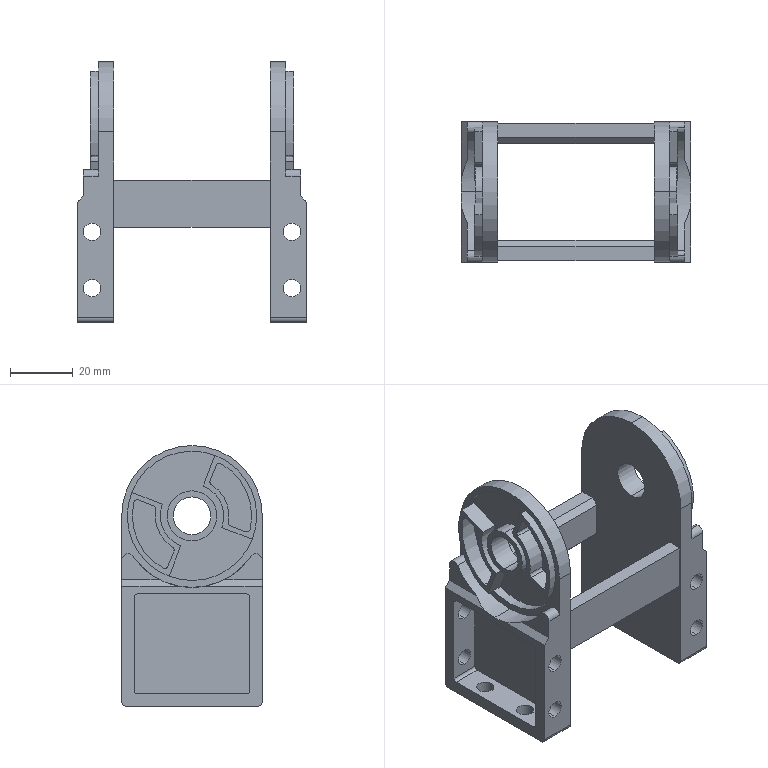Part | SolidWorks | features BaseBody 1 | 1 solid | 168 faces | box 73.47 x 44.999 x 83.497 mm | volume 40679 mm3 | cylinder 98 | plane 70 | commonest cylinder face diameters 2 x28 5.5 x24 41.398 x10 4 x6 3 x4 12.1 x4